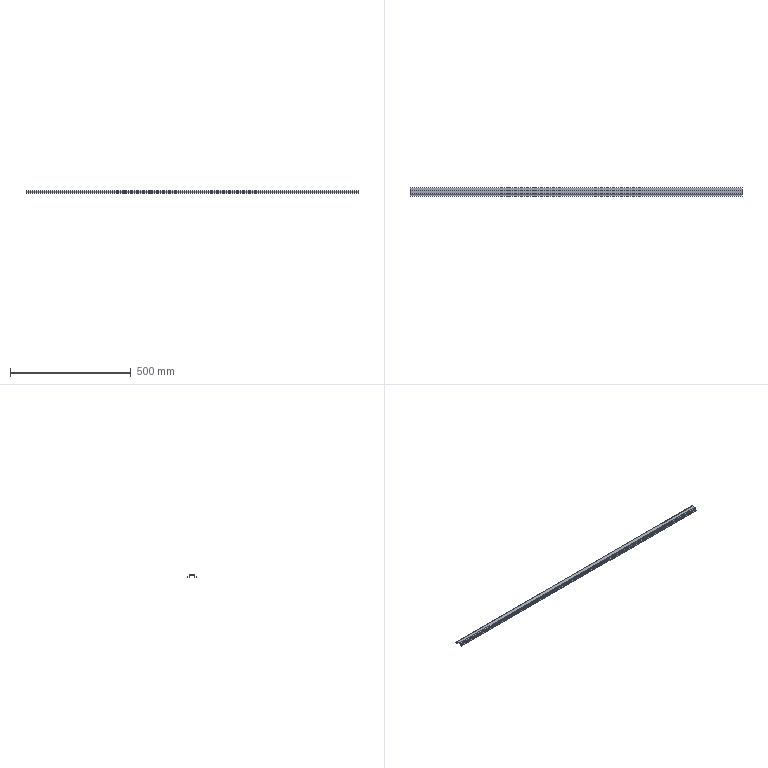Part | SolidWorks | features EdgeFlange 2, FlatPattern 1, SMBaseFlange 1, SheetMetal 1 | 1 solid | 38 faces | box 1375 x 34 x 11 mm | volume 101345 mm3 | plane 30 | cylinder 8 | commonest cylinder face diameters 3 x4 6 x4
STEP:
#1=CARTESIAN_POINT('',(687.5,-7.5,0.));
#2=VERTEX_POINT('',#1);
#3=CARTESIAN_POINT('',(687.5,7.5,0.));
#4=VERTEX_POINT('',#3);
#5=CARTESIAN_POINT('',(687.5,-7.5,0.));
#6=DIRECTION('',(0.,1.,0.));
#7=VECTOR('',#6,1000.);
#8=LINE('',#5,#7);
#9=EDGE_CURVE('',#2,#4,#8,.T.);
#10=ORIENTED_EDGE('',*,*,#9,.F.);
#11=CARTESIAN_POINT('',(687.5,-7.5,-1.5));
#12=VERTEX_POINT('',#11);
#13=CARTESIAN_POINT('',(687.5,-7.5,-1.5));
#14=DIRECTION('',(0.,0.,1.));
#15=VECTOR('',#14,1000.);
#16=LINE('',#13,#15);
#17=EDGE_CURVE('',#12,#2,#16,.T.);
#18=ORIENTED_EDGE('',*,*,#17,.F.);
#19=CARTESIAN_POINT('',(687.5,7.5,-1.5));
#20=VERTEX_POINT('',#19);
#21=CARTESIAN_POINT('',(687.5,-7.5,-1.5));
#22=DIRECTION('',(0.,1.,0.));
#23=VECTOR('',#22,1000.);
#24=LINE('',#21,#23);
#25=EDGE_CURVE('',#12,#20,#24,.T.);
#26=ORIENTED_EDGE('',*,*,#25,.T.);
#27=CARTESIAN_POINT('',(687.5,7.5,-1.5));
#28=DIRECTION('',(0.,0.,1.));
#29=VECTOR('',#28,1000.);
#30=LINE('',#27,#29);
#31=EDGE_CURVE('',#20,#4,#30,.T.);
#32=ORIENTED_EDGE('',*,*,#31,.T.);
#33=EDGE_LOOP('',(#10,#18,#26,#32));
#34=FACE_OUTER_BOUND('',#33,.T.);
#35=CARTESIAN_POINT('',(687.5,-7.5,-1.5));
#36=DIRECTION('',(1.,0.,0.));
#37=DIRECTION('',(0.,0.,-1.));
#38=AXIS2_PLACEMENT_3D('',#35,#36,#37);
#39=PLANE('',#38);
#40=ADVANCED_FACE('',(#34),#39,.T.);
#41=CARTESIAN_POINT('',(-687.5,7.5,0.));
#42=VERTEX_POINT('',#41);
#43=CARTESIAN_POINT('',(-687.5,-7.5,0.));
#44=VERTEX_POINT('',#43);
#45=CARTESIAN_POINT('',(-687.5,-7.5,0.));
#46=DIRECTION('',(0.,-1.,0.));
#47=VECTOR('',#46,1000.);
#48=LINE('',#45,#47);
#49=EDGE_CURVE('',#42,#44,#48,.T.);
#50=ORIENTED_EDGE('',*,*,#49,.F.);
#51=CARTESIAN_POINT('',(-687.5,7.5,-1.5));
#52=VERTEX_POINT('',#51);
#53=CARTESIAN_POINT('',(-687.5,7.5,-1.5));
#54=DIRECTION('',(0.,0.,1.));
#55=VECTOR('',#54,1000.);
#56=LINE('',#53,#55);
#57=EDGE_CURVE('',#52,#42,#56,.T.);
#58=ORIENTED_EDGE('',*,*,#57,.F.);
#59=CARTESIAN_POINT('',(-687.5,-7.5,-1.5));
#60=VERTEX_POINT('',#59);
#61=CARTESIAN_POINT('',(-687.5,-7.5,-1.5));
#62=DIRECTION('',(0.,-1.,0.));
#63=VECTOR('',#62,1000.);
#64=LINE('',#61,#63);
#65=EDGE_CURVE('',#52,#60,#64,.T.);
#66=ORIENTED_EDGE('',*,*,#65,.T.);
#67=CARTESIAN_POINT('',(-687.5,-7.5,-1.5));
#68=DIRECTION('',(0.,0.,1.));
#69=VECTOR('',#68,1000.);
#70=LINE('',#67,#69);
#71=EDGE_CURVE('',#60,#44,#70,.T.);
#72=ORIENTED_EDGE('',*,*,#71,.T.);
#73=EDGE_LOOP('',(#50,#58,#66,#72));
#74=FACE_OUTER_BOUND('',#73,.T.);
#75=CARTESIAN_POINT('',(-687.5,-7.5,-1.5));
#76=DIRECTION('',(-1.,0.,0.));
#77=DIRECTION('',(0.,0.,1.));
#78=AXIS2_PLACEMENT_3D('',#75,#76,#77);
#79=PLANE('',#78);
#80=ADVANCED_FACE('',(#74),#79,.T.);
#81=ORIENTED_EDGE('',*,*,#25,.F.);
#82=CARTESIAN_POINT('',(-687.5,-7.5,-1.5));
#83=DIRECTION('',(1.,0.,0.));
#84=VECTOR('',#83,1000.);
#85=LINE('',#82,#84);
#86=EDGE_CURVE('',#60,#12,#85,.T.);
#87=ORIENTED_EDGE('',*,*,#86,.F.);
#88=ORIENTED_EDGE('',*,*,#65,.F.);
#89=CARTESIAN_POINT('',(-687.5,7.5,-1.5));
#90=DIRECTION('',(-1.,0.,0.));
#91=VECTOR('',#90,1000.);
#92=LINE('',#89,#91);
#93=EDGE_CURVE('',#20,#52,#92,.T.);
#94=ORIENTED_EDGE('',*,*,#93,.F.);
#95=EDGE_LOOP('',(#81,#87,#88,#94));
#96=FACE_OUTER_BOUND('',#95,.T.);
#97=CARTESIAN_POINT('',(0.,0.,-1.5));
#98=DIRECTION('',(0.,0.,-1.));
#99=DIRECTION('',(-1.,0.,0.));
#100=AXIS2_PLACEMENT_3D('',#97,#98,#99);
#101=PLANE('',#100);
#102=ADVANCED_FACE('',(#96),#101,.T.);
#103=ORIENTED_EDGE('',*,*,#9,.T.);
#104=CARTESIAN_POINT('',(-687.5,7.5,0.));
#105=DIRECTION('',(-1.,0.,0.));
#106=VECTOR('',#105,1000.);
#107=LINE('',#104,#106);
#108=EDGE_CURVE('',#4,#42,#107,.T.);
#109=ORIENTED_EDGE('',*,*,#108,.T.);
#110=ORIENTED_EDGE('',*,*,#49,.T.);
#111=CARTESIAN_POINT('',(-687.5,-7.5,0.));
#112=DIRECTION('',(1.,0.,0.));
#113=VECTOR('',#112,1000.);
#114=LINE('',#111,#113);
#115=EDGE_CURVE('',#44,#2,#114,.T.);
#116=ORIENTED_EDGE('',*,*,#115,.T.);
#117=EDGE_LOOP('',(#103,#109,#110,#116));
#118=FACE_OUTER_BOUND('',#117,.T.);
#119=CARTESIAN_POINT('',(0.,0.,0.));
#120=DIRECTION('',(0.,0.,-1.));
#121=DIRECTION('',(-1.,0.,0.));
#122=AXIS2_PLACEMENT_3D('',#119,#120,#121);
#123=PLANE('',#122);
#124=ADVANCED_FACE('',(#118),#123,.F.);
#125=CARTESIAN_POINT('',(-687.5,9.,-3.));
#126=VERTEX_POINT('',#125);
#127=CARTESIAN_POINT('',(-687.5,10.5,-3.));
#128=VERTEX_POINT('',#127);
#129=CARTESIAN_POINT('',(-687.5,10.5,-3.));
#130=DIRECTION('',(0.,1.,0.));
#131=VECTOR('',#130,1000.);
#132=LINE('',#129,#131);
#133=EDGE_CURVE('',#126,#128,#132,.T.);
#134=ORIENTED_EDGE('',*,*,#133,.F.);
#135=CARTESIAN_POINT('',(-687.5,7.5,-3.));
#136=DIRECTION('',(-1.,0.,0.));
#137=DIRECTION('',(0.,0.,-1.));
#138=AXIS2_PLACEMENT_3D('',#135,#136,#137);
#139=CIRCLE('',#138,1.5);
#140=EDGE_CURVE('',#52,#126,#139,.T.);
#141=ORIENTED_EDGE('',*,*,#140,.F.);
#142=ORIENTED_EDGE('',*,*,#57,.T.);
#143=CARTESIAN_POINT('',(-687.5,7.5,-3.));
#144=DIRECTION('',(-1.,0.,0.));
#145=DIRECTION('',(0.,0.,-1.));
#146=AXIS2_PLACEMENT_3D('',#143,#144,#145);
#147=CIRCLE('',#146,3.);
#148=EDGE_CURVE('',#42,#128,#147,.T.);
#149=ORIENTED_EDGE('',*,*,#148,.T.);
#150=EDGE_LOOP('',(#134,#141,#142,#149));
#151=FACE_OUTER_BOUND('',#150,.T.);
#152=CARTESIAN_POINT('',(-687.5,7.5,-3.));
#153=DIRECTION('',(-1.,0.,0.));
#154=DIRECTION('',(0.,0.,1.));
#155=AXIS2_PLACEMENT_3D('',#152,#153,#154);
#156=PLANE('',#155);
#157=ADVANCED_FACE('',(#151),#156,.T.);
#158=CARTESIAN_POINT('',(687.5,9.,-3.));
#159=VERTEX_POINT('',#158);
#160=CARTESIAN_POINT('',(687.5,7.5,-3.));
#161=DIRECTION('',(1.,0.,0.));
#162=DIRECTION('',(0.,0.,-1.));
#163=AXIS2_PLACEMENT_3D('',#160,#161,#162);
#164=CIRCLE('',#163,1.5);
#165=EDGE_CURVE('',#159,#20,#164,.T.);
#166=ORIENTED_EDGE('',*,*,#165,.F.);
#167=CARTESIAN_POINT('',(687.5,10.5,-3.));
#168=VERTEX_POINT('',#167);
#169=CARTESIAN_POINT('',(687.5,9.,-3.));
#170=DIRECTION('',(0.,1.,0.));
#171=VECTOR('',#170,1000.);
#172=LINE('',#169,#171);
#173=EDGE_CURVE('',#159,#168,#172,.T.);
#174=ORIENTED_EDGE('',*,*,#173,.T.);
#175=CARTESIAN_POINT('',(687.5,7.5,-3.));
#176=DIRECTION('',(1.,0.,0.));
#177=DIRECTION('',(0.,0.,-1.));
#178=AXIS2_PLACEMENT_3D('',#175,#176,#177);
#179=CIRCLE('',#178,3.);
#180=EDGE_CURVE('',#168,#4,#179,.T.);
#181=ORIENTED_EDGE('',*,*,#180,.T.);
#182=ORIENTED_EDGE('',*,*,#31,.F.);
#183=EDGE_LOOP('',(#166,#174,#181,#182));
#184=FACE_OUTER_BOUND('',#183,.T.);
#185=CARTESIAN_POINT('',(687.5,7.5,-3.));
#186=DIRECTION('',(-1.,0.,0.));
#187=DIRECTION('',(0.,0.,1.));
#188=AXIS2_PLACEMENT_3D('',#185,#186,#187);
#189=PLANE('',#188);
#190=ADVANCED_FACE('',(#184),#189,.F.);
#191=ORIENTED_EDGE('',*,*,#108,.F.);
#192=ORIENTED_EDGE('',*,*,#180,.F.);
#193=CARTESIAN_POINT('',(-687.5,10.5,-3.));
#194=DIRECTION('',(-1.,0.,0.));
#195=VECTOR('',#194,1000.);
#196=LINE('',#193,#195);
#197=EDGE_CURVE('',#168,#128,#196,.T.);
#198=ORIENTED_EDGE('',*,*,#197,.T.);
#199=ORIENTED_EDGE('',*,*,#148,.F.);
#200=EDGE_LOOP('',(#191,#192,#198,#199));
#201=FACE_OUTER_BOUND('',#200,.T.);
#202=CARTESIAN_POINT('',(687.5,7.5,-3.));
#203=DIRECTION('',(1.,0.,0.));
#204=DIRECTION('',(0.,1.,0.));
#205=AXIS2_PLACEMENT_3D('',#202,#203,#204);
#206=CYLINDRICAL_SURFACE('',#205,3.);
#207=ADVANCED_FACE('',(#201),#206,.T.);
#208=ORIENTED_EDGE('',*,*,#93,.T.);
#209=ORIENTED_EDGE('',*,*,#140,.T.);
#210=CARTESIAN_POINT('',(-687.5,9.,-3.));
#211=DIRECTION('',(1.,0.,0.));
#212=VECTOR('',#211,1000.);
#213=LINE('',#210,#212);
#214=EDGE_CURVE('',#126,#159,#213,.T.);
#215=ORIENTED_EDGE('',*,*,#214,.T.);
#216=ORIENTED_EDGE('',*,*,#165,.T.);
#217=EDGE_LOOP('',(#208,#209,#215,#216));
#218=FACE_OUTER_BOUND('',#217,.T.);
#219=CARTESIAN_POINT('',(687.5,7.5,-3.));
#220=DIRECTION('',(1.,0.,0.));
#221=DIRECTION('',(0.,1.,0.));
#222=AXIS2_PLACEMENT_3D('',#219,#220,#221);
#223=CYLINDRICAL_SURFACE('',#222,1.5);
#224=ADVANCED_FACE('',(#218),#223,.F.);
#225=ORIENTED_EDGE('',*,*,#173,.F.);
#226=CARTESIAN_POINT('',(687.5,9.,-8.));
#227=VERTEX_POINT('',#226);
#228=CARTESIAN_POINT('',(687.5,9.,-8.));
#229=DIRECTION('',(0.,0.,-1.));
#230=VECTOR('',#229,1000.);
#231=LINE('',#228,#230);
#232=EDGE_CURVE('',#159,#227,#231,.T.);
#233=ORIENTED_EDGE('',*,*,#232,.T.);
#234=CARTESIAN_POINT('',(687.5,10.5,-8.));
#235=VERTEX_POINT('',#234);
#236=CARTESIAN_POINT('',(687.5,10.5,-8.));
#237=DIRECTION('',(0.,-1.,0.));
#238=VECTOR('',#237,1000.);
#239=LINE('',#236,#238);
#240=EDGE_CURVE('',#235,#227,#239,.T.);
#241=ORIENTED_EDGE('',*,*,#240,.F.);
#242=CARTESIAN_POINT('',(687.5,10.5,0.));
#243=DIRECTION('',(0.,0.,-1.));
#244=VECTOR('',#243,1000.);
#245=LINE('',#242,#244);
#246=EDGE_CURVE('',#168,#235,#245,.T.);
#247=ORIENTED_EDGE('',*,*,#246,.F.);
#248=EDGE_LOOP('',(#225,#233,#241,#247));
#249=FACE_OUTER_BOUND('',#248,.T.);
#250=CARTESIAN_POINT('',(687.5,10.5,-8.));
#251=DIRECTION('',(-1.,0.,0.));
#252=DIRECTION('',(0.,0.,1.));
#253=AXIS2_PLACEMENT_3D('',#250,#251,#252);
#254=PLANE('',#253);
#255=ADVANCED_FACE('',(#249),#254,.F.);
#256=ORIENTED_EDGE('',*,*,#133,.T.);
#257=CARTESIAN_POINT('',(-687.5,10.5,-8.));
#258=VERTEX_POINT('',#257);
#259=CARTESIAN_POINT('',(-687.5,10.5,0.));
#260=DIRECTION('',(0.,0.,1.));
#261=VECTOR('',#260,1000.);
#262=LINE('',#259,#261);
#263=EDGE_CURVE('',#258,#128,#262,.T.);
#264=ORIENTED_EDGE('',*,*,#263,.F.);
#265=CARTESIAN_POINT('',(-687.5,9.,-8.));
#266=VERTEX_POINT('',#265);
#267=CARTESIAN_POINT('',(-687.5,10.5,-8.));
#268=DIRECTION('',(0.,-1.,0.));
#269=VECTOR('',#268,1000.);
#270=LINE('',#267,#269);
#271=EDGE_CURVE('',#258,#266,#270,.T.);
#272=ORIENTED_EDGE('',*,*,#271,.T.);
#273=CARTESIAN_POINT('',(-687.5,9.,-1.5));
#274=DIRECTION('',(0.,0.,1.));
#275=VECTOR('',#274,1000.);
#276=LINE('',#273,#275);
#277=EDGE_CURVE('',#266,#126,#276,.T.);
#278=ORIENTED_EDGE('',*,*,#277,.T.);
#279=EDGE_LOOP('',(#256,#264,#272,#278));
#280=FACE_OUTER_BOUND('',#279,.T.);
#281=CARTESIAN_POINT('',(-687.5,10.5,-1.5));
#282=DIRECTION('',(1.,0.,0.));
#283=DIRECTION('',(0.,0.,-1.));
#284=AXIS2_PLACEMENT_3D('',#281,#282,#283);
#285=PLANE('',#284);
#286=ADVANCED_FACE('',(#280),#285,.F.);
#287=ORIENTED_EDGE('',*,*,#197,.F.);
#288=ORIENTED_EDGE('',*,*,#246,.T.);
#289=CARTESIAN_POINT('',(0.,10.5,-8.));
#290=DIRECTION('',(-1.,0.,0.));
#291=VECTOR('',#290,1000.);
#292=LINE('',#289,#291);
#293=EDGE_CURVE('',#235,#258,#292,.T.);
#294=ORIENTED_EDGE('',*,*,#293,.T.);
#295=ORIENTED_EDGE('',*,*,#263,.T.);
#296=EDGE_LOOP('',(#287,#288,#294,#295));
#297=FACE_OUTER_BOUND('',#296,.T.);
#298=CARTESIAN_POINT('',(0.,10.5,0.));
#299=DIRECTION('',(0.,-1.,0.));
#300=DIRECTION('',(0.,0.,-1.));
#301=AXIS2_PLACEMENT_3D('',#298,#299,#300);
#302=PLANE('',#301);
#303=ADVANCED_FACE('',(#297),#302,.F.);
#304=ORIENTED_EDGE('',*,*,#232,.F.);
#305=ORIENTED_EDGE('',*,*,#214,.F.);
#306=ORIENTED_EDGE('',*,*,#277,.F.);
#307=CARTESIAN_POINT('',(-687.5,9.,-8.));
#308=DIRECTION('',(-1.,0.,0.));
#309=VECTOR('',#308,1000.);
#310=LINE('',#307,#309);
#311=EDGE_CURVE('',#227,#266,#310,.T.);
#312=ORIENTED_EDGE('',*,*,#311,.F.);
#313=EDGE_LOOP('',(#304,#305,#306,#312));
#314=FACE_OUTER_BOUND('',#313,.T.);
#315=CARTESIAN_POINT('',(0.,9.,0.));
#316=DIRECTION('',(0.,-1.,0.));
#317=DIRECTION('',(0.,0.,-1.));
#318=AXIS2_PLACEMENT_3D('',#315,#316,#317);
#319=PLANE('',#318);
#320=ADVANCED_FACE('',(#314),#319,.T.);
#321=CARTESIAN_POINT('',(687.5,-9.,-3.));
#322=VERTEX_POINT('',#321);
#323=CARTESIAN_POINT('',(687.5,-10.5,-3.));
#324=VERTEX_POINT('',#323);
#325=CARTESIAN_POINT('',(687.5,-10.5,-3.));
#326=DIRECTION('',(0.,-1.,0.));
#327=VECTOR('',#326,1000.);
#328=LINE('',#325,#327);
#329=EDGE_CURVE('',#322,#324,#328,.T.);
#330=ORIENTED_EDGE('',*,*,#329,.F.);
#331=CARTESIAN_POINT('',(687.5,-7.5,-3.));
#332=DIRECTION('',(1.,0.,0.));
#333=DIRECTION('',(0.,0.,1.));
#334=AXIS2_PLACEMENT_3D('',#331,#332,#333);
#335=CIRCLE('',#334,1.5);
#336=EDGE_CURVE('',#12,#322,#335,.T.);
#337=ORIENTED_EDGE('',*,*,#336,.F.);
#338=ORIENTED_EDGE('',*,*,#17,.T.);
#339=CARTESIAN_POINT('',(687.5,-7.5,-3.));
#340=DIRECTION('',(1.,0.,0.));
#341=DIRECTION('',(0.,0.,1.));
#342=AXIS2_PLACEMENT_3D('',#339,#340,#341);
#343=CIRCLE('',#342,3.);
#344=EDGE_CURVE('',#2,#324,#343,.T.);
#345=ORIENTED_EDGE('',*,*,#344,.T.);
#346=EDGE_LOOP('',(#330,#337,#338,#345));
#347=FACE_OUTER_BOUND('',#346,.T.);
#348=CARTESIAN_POINT('',(687.5,-7.5,-3.));
#349=DIRECTION('',(1.,0.,0.));
#350=DIRECTION('',(0.,0.,-1.));
#351=AXIS2_PLACEMENT_3D('',#348,#349,#350);
#352=PLANE('',#351);
#353=ADVANCED_FACE('',(#347),#352,.T.);
#354=CARTESIAN_POINT('',(-687.5,-9.,-3.));
#355=VERTEX_POINT('',#354);
#356=CARTESIAN_POINT('',(-687.5,-7.5,-3.));
#357=DIRECTION('',(-1.,0.,0.));
#358=DIRECTION('',(0.,0.,1.));
#359=AXIS2_PLACEMENT_3D('',#356,#357,#358);
#360=CIRCLE('',#359,1.5);
#361=EDGE_CURVE('',#355,#60,#360,.T.);
#362=ORIENTED_EDGE('',*,*,#361,.F.);
#363=CARTESIAN_POINT('',(-687.5,-10.5,-3.));
#364=VERTEX_POINT('',#363);
#365=CARTESIAN_POINT('',(-687.5,-9.,-3.));
#366=DIRECTION('',(0.,-1.,0.));
#367=VECTOR('',#366,1000.);
#368=LINE('',#365,#367);
#369=EDGE_CURVE('',#355,#364,#368,.T.);
#370=ORIENTED_EDGE('',*,*,#369,.T.);
#371=CARTESIAN_POINT('',(-687.5,-7.5,-3.));
#372=DIRECTION('',(-1.,0.,0.));
#373=DIRECTION('',(0.,0.,1.));
#374=AXIS2_PLACEMENT_3D('',#371,#372,#373);
#375=CIRCLE('',#374,3.);
#376=EDGE_CURVE('',#364,#44,#375,.T.);
#377=ORIENTED_EDGE('',*,*,#376,.T.);
#378=ORIENTED_EDGE('',*,*,#71,.F.);
#379=EDGE_LOOP('',(#362,#370,#377,#378));
#380=FACE_OUTER_BOUND('',#379,.T.);
#381=CARTESIAN_POINT('',(-687.5,-7.5,-3.));
#382=DIRECTION('',(1.,0.,0.));
#383=DIRECTION('',(0.,0.,-1.));
#384=AXIS2_PLACEMENT_3D('',#381,#382,#383);
#385=PLANE('',#384);
#386=ADVANCED_FACE('',(#380),#385,.F.);
#387=ORIENTED_EDGE('',*,*,#115,.F.);
#388=ORIENTED_EDGE('',*,*,#376,.F.);
#389=CARTESIAN_POINT('',(687.5,-10.5,-3.));
#390=DIRECTION('',(1.,0.,0.));
#391=VECTOR('',#390,1000.);
#392=LINE('',#389,#391);
#393=EDGE_CURVE('',#364,#324,#392,.T.);
#394=ORIENTED_EDGE('',*,*,#393,.T.);
#395=ORIENTED_EDGE('',*,*,#344,.F.);
#396=EDGE_LOOP('',(#387,#388,#394,#395));
#397=FACE_OUTER_BOUND('',#396,.T.);
#398=CARTESIAN_POINT('',(-687.5,-7.5,-3.));
#399=DIRECTION('',(-1.,0.,0.));
#400=DIRECTION('',(0.,-1.,0.));
#401=AXIS2_PLACEMENT_3D('',#398,#399,#400);
#402=CYLINDRICAL_SURFACE('',#401,3.);
#403=ADVANCED_FACE('',(#397),#402,.T.);
#404=ORIENTED_EDGE('',*,*,#86,.T.);
#405=ORIENTED_EDGE('',*,*,#336,.T.);
#406=CARTESIAN_POINT('',(687.5,-9.,-3.));
#407=DIRECTION('',(-1.,0.,0.));
#408=VECTOR('',#407,1000.);
#409=LINE('',#406,#408);
#410=EDGE_CURVE('',#322,#355,#409,.T.);
#411=ORIENTED_EDGE('',*,*,#410,.T.);
#412=ORIENTED_EDGE('',*,*,#361,.T.);
#413=EDGE_LOOP('',(#404,#405,#411,#412));
#414=FACE_OUTER_BOUND('',#413,.T.);
#415=CARTESIAN_POINT('',(-687.5,-7.5,-3.));
#416=DIRECTION('',(-1.,0.,0.));
#417=DIRECTION('',(0.,-1.,0.));
#418=AXIS2_PLACEMENT_3D('',#415,#416,#417);
#419=CYLINDRICAL_SURFACE('',#418,1.5);
#420=ADVANCED_FACE('',(#414),#419,.F.);
#421=ORIENTED_EDGE('',*,*,#369,.F.);
#422=CARTESIAN_POINT('',(-687.5,-9.,-8.));
#423=VERTEX_POINT('',#422);
#424=CARTESIAN_POINT('',(-687.5,-9.,-8.));
#425=DIRECTION('',(0.,0.,-1.));
#426=VECTOR('',#425,1000.);
#427=LINE('',#424,#426);
#428=EDGE_CURVE('',#355,#423,#427,.T.);
#429=ORIENTED_EDGE('',*,*,#428,.T.);
#430=CARTESIAN_POINT('',(-687.5,-10.5,-8.));
#431=VERTEX_POINT('',#430);
#432=CARTESIAN_POINT('',(-687.5,-10.5,-8.));
#433=DIRECTION('',(0.,1.,0.));
#434=VECTOR('',#433,1000.);
#435=LINE('',#432,#434);
#436=EDGE_CURVE('',#431,#423,#435,.T.);
#437=ORIENTED_EDGE('',*,*,#436,.F.);
#438=CARTESIAN_POINT('',(-687.5,-10.5,0.));
#439=DIRECTION('',(0.,0.,-1.));
#440=VECTOR('',#439,1000.);
#441=LINE('',#438,#440);
#442=EDGE_CURVE('',#364,#431,#441,.T.);
#443=ORIENTED_EDGE('',*,*,#442,.F.);
#444=EDGE_LOOP('',(#421,#429,#437,#443));
#445=FACE_OUTER_BOUND('',#444,.T.);
#446=CARTESIAN_POINT('',(-687.5,-10.5,-8.));
#447=DIRECTION('',(1.,0.,0.));
#448=DIRECTION('',(0.,0.,-1.));
#449=AXIS2_PLACEMENT_3D('',#446,#447,#448);
#450=PLANE('',#449);
#451=ADVANCED_FACE('',(#445),#450,.F.);
#452=ORIENTED_EDGE('',*,*,#329,.T.);
#453=CARTESIAN_POINT('',(687.5,-10.5,-8.));
#454=VERTEX_POINT('',#453);
#455=CARTESIAN_POINT('',(687.5,-10.5,0.));
#456=DIRECTION('',(0.,0.,1.));
#457=VECTOR('',#456,1000.);
#458=LINE('',#455,#457);
#459=EDGE_CURVE('',#454,#324,#458,.T.);
#460=ORIENTED_EDGE('',*,*,#459,.F.);
#461=CARTESIAN_POINT('',(687.5,-9.,-8.));
#462=VERTEX_POINT('',#461);
#463=CARTESIAN_POINT('',(687.5,-10.5,-8.));
#464=DIRECTION('',(0.,1.,0.));
#465=VECTOR('',#464,1000.);
#466=LINE('',#463,#465);
#467=EDGE_CURVE('',#454,#462,#466,.T.);
#468=ORIENTED_EDGE('',*,*,#467,.T.);
#469=CARTESIAN_POINT('',(687.5,-9.,-1.5));
#470=DIRECTION('',(0.,0.,1.));
#471=VECTOR('',#470,1000.);
#472=LINE('',#469,#471);
#473=EDGE_CURVE('',#462,#322,#472,.T.);
#474=ORIENTED_EDGE('',*,*,#473,.T.);
#475=EDGE_LOOP('',(#452,#460,#468,#474));
#476=FACE_OUTER_BOUND('',#475,.T.);
#477=CARTESIAN_POINT('',(687.5,-10.5,-1.5));
#478=DIRECTION('',(-1.,0.,0.));
#479=DIRECTION('',(0.,0.,1.));
#480=AXIS2_PLACEMENT_3D('',#477,#478,#479);
#481=PLANE('',#480);
#482=ADVANCED_FACE('',(#476),#481,.F.);
#483=ORIENTED_EDGE('',*,*,#393,.F.);
#484=ORIENTED_EDGE('',*,*,#442,.T.);
#485=CARTESIAN_POINT('',(0.,-10.5,-8.));
#486=DIRECTION('',(1.,0.,0.));
#487=VECTOR('',#486,1000.);
#488=LINE('',#485,#487);
#489=EDGE_CURVE('',#431,#454,#488,.T.);
#490=ORIENTED_EDGE('',*,*,#489,.T.);
#491=ORIENTED_EDGE('',*,*,#459,.T.);
#492=EDGE_LOOP('',(#483,#484,#490,#491));
#493=FACE_OUTER_BOUND('',#492,.T.);
#494=CARTESIAN_POINT('',(0.,-10.5,0.));
#495=DIRECTION('',(0.,1.,0.));
#496=DIRECTION('',(0.,0.,1.));
#497=AXIS2_PLACEMENT_3D('',#494,#495,#496);
#498=PLANE('',#497);
#499=ADVANCED_FACE('',(#493),#498,.F.);
#500=ORIENTED_EDGE('',*,*,#428,.F.);
#501=ORIENTED_EDGE('',*,*,#410,.F.);
#502=ORIENTED_EDGE('',*,*,#473,.F.);
#503=CARTESIAN_POINT('',(687.5,-9.,-8.));
#504=DIRECTION('',(1.,0.,0.));
#505=VECTOR('',#504,1000.);
#506=LINE('',#503,#505);
#507=EDGE_CURVE('',#423,#462,#506,.T.);
#508=ORIENTED_EDGE('',*,*,#507,.F.);
#509=EDGE_LOOP('',(#500,#501,#502,#508));
#510=FACE_OUTER_BOUND('',#509,.T.);
#511=CARTESIAN_POINT('',(0.,-9.,0.));
#512=DIRECTION('',(0.,1.,0.));
#513=DIRECTION('',(0.,0.,1.));
#514=AXIS2_PLACEMENT_3D('',#511,#512,#513);
#515=PLANE('',#514);
#516=ADVANCED_FACE('',(#510),#515,.T.);
#517=CARTESIAN_POINT('',(687.5,12.,-9.5));
#518=VERTEX_POINT('',#517);
#519=CARTESIAN_POINT('',(687.5,12.,-11.));
#520=VERTEX_POINT('',#519);
#521=CARTESIAN_POINT('',(687.5,12.,-11.));
#522=DIRECTION('',(0.,0.,-1.));
#523=VECTOR('',#522,1000.);
#524=LINE('',#521,#523);
#525=EDGE_CURVE('',#518,#520,#524,.T.);
#526=ORIENTED_EDGE('',*,*,#525,.F.);
#527=CARTESIAN_POINT('',(687.5,12.,-8.));
#528=DIRECTION('',(1.,0.,0.));
#529=DIRECTION('',(0.,0.,1.));
#530=AXIS2_PLACEMENT_3D('',#527,#528,#529);
#531=CIRCLE('',#530,1.5);
#532=EDGE_CURVE('',#235,#518,#531,.T.);
#533=ORIENTED_EDGE('',*,*,#532,.F.);
#534=ORIENTED_EDGE('',*,*,#240,.T.);
#535=CARTESIAN_POINT('',(687.5,12.,-8.));
#536=DIRECTION('',(1.,0.,0.));
#537=DIRECTION('',(0.,0.,1.));
#538=AXIS2_PLACEMENT_3D('',#535,#536,#537);
#539=CIRCLE('',#538,3.);
#540=EDGE_CURVE('',#227,#520,#539,.T.);
#541=ORIENTED_EDGE('',*,*,#540,.T.);
#542=EDGE_LOOP('',(#526,#533,#534,#541));
#543=FACE_OUTER_BOUND('',#542,.T.);
#544=CARTESIAN_POINT('',(687.5,12.,-8.));
#545=DIRECTION('',(1.,0.,0.));
#546=DIRECTION('',(0.,0.,-1.));
#547=AXIS2_PLACEMENT_3D('',#544,#545,#546);
#548=PLANE('',#547);
#549=ADVANCED_FACE('',(#543),#548,.T.);
#550=CARTESIAN_POINT('',(-687.5,12.,-9.5));
#551=VERTEX_POINT('',#550);
#552=CARTESIAN_POINT('',(-687.5,12.,-8.));
#553=DIRECTION('',(-1.,0.,0.));
#554=DIRECTION('',(0.,0.,1.));
#555=AXIS2_PLACEMENT_3D('',#552,#553,#554);
#556=CIRCLE('',#555,1.5);
#557=EDGE_CURVE('',#551,#258,#556,.T.);
#558=ORIENTED_EDGE('',*,*,#557,.F.);
#559=CARTESIAN_POINT('',(-687.5,12.,-11.));
#560=VERTEX_POINT('',#559);
#561=CARTESIAN_POINT('',(-687.5,12.,-9.5));
#562=DIRECTION('',(0.,0.,-1.));
#563=VECTOR('',#562,1000.);
#564=LINE('',#561,#563);
#565=EDGE_CURVE('',#551,#560,#564,.T.);
#566=ORIENTED_EDGE('',*,*,#565,.T.);
#567=CARTESIAN_POINT('',(-687.5,12.,-8.));
#568=DIRECTION('',(-1.,0.,0.));
#569=DIRECTION('',(0.,0.,1.));
#570=AXIS2_PLACEMENT_3D('',#567,#568,#569);
#571=CIRCLE('',#570,3.);
#572=EDGE_CURVE('',#560,#266,#571,.T.);
#573=ORIENTED_EDGE('',*,*,#572,.T.);
#574=ORIENTED_EDGE('',*,*,#271,.F.);
#575=EDGE_LOOP('',(#558,#566,#573,#574));
#576=FACE_OUTER_BOUND('',#575,.T.);
#577=CARTESIAN_POINT('',(-687.5,12.,-8.));
#578=DIRECTION('',(1.,0.,0.));
#579=DIRECTION('',(0.,0.,-1.));
#580=AXIS2_PLACEMENT_3D('',#577,#578,#579);
#581=PLANE('',#580);
#582=ADVANCED_FACE('',(#576),#581,.F.);
#583=ORIENTED_EDGE('',*,*,#311,.T.);
#584=ORIENTED_EDGE('',*,*,#572,.F.);
#585=CARTESIAN_POINT('',(0.,12.,-11.));
#586=DIRECTION('',(-1.,0.,0.));
#587=VECTOR('',#586,1000.);
#588=LINE('',#585,#587);
#589=EDGE_CURVE('',#520,#560,#588,.T.);
#590=ORIENTED_EDGE('',*,*,#589,.F.);
#591=ORIENTED_EDGE('',*,*,#540,.F.);
#592=EDGE_LOOP('',(#583,#584,#590,#591));
#593=FACE_OUTER_BOUND('',#592,.T.);
#594=CARTESIAN_POINT('',(-687.5,12.,-8.));
#595=DIRECTION('',(-1.,0.,0.));
#596=DIRECTION('',(0.,0.,-1.));
#597=AXIS2_PLACEMENT_3D('',#594,#595,#596);
#598=CYLINDRICAL_SURFACE('',#597,3.);
#599=ADVANCED_FACE('',(#593),#598,.T.);
#600=ORIENTED_EDGE('',*,*,#293,.F.);
#601=ORIENTED_EDGE('',*,*,#532,.T.);
#602=CARTESIAN_POINT('',(687.5,12.,-9.5));
#603=DIRECTION('',(-1.,0.,0.));
#604=VECTOR('',#603,1000.);
#605=LINE('',#602,#604);
#606=EDGE_CURVE('',#518,#551,#605,.T.);
#607=ORIENTED_EDGE('',*,*,#606,.T.);
#608=ORIENTED_EDGE('',*,*,#557,.T.);
#609=EDGE_LOOP('',(#600,#601,#607,#608));
#610=FACE_OUTER_BOUND('',#609,.T.);
#611=CARTESIAN_POINT('',(-687.5,12.,-8.));
#612=DIRECTION('',(-1.,0.,0.));
#613=DIRECTION('',(0.,0.,-1.));
#614=AXIS2_PLACEMENT_3D('',#611,#612,#613);
#615=CYLINDRICAL_SURFACE('',#614,1.5);
#616=ADVANCED_FACE('',(#610),#615,.F.);
#617=CARTESIAN_POINT('',(-687.5,17.,-11.));
#618=VERTEX_POINT('',#617);
#619=CARTESIAN_POINT('',(-687.5,10.5,-11.));
#620=DIRECTION('',(0.,-1.,0.));
#621=VECTOR('',#620,1000.);
#622=LINE('',#619,#621);
#623=EDGE_CURVE('',#618,#560,#622,.T.);
#624=ORIENTED_EDGE('',*,*,#623,.T.);
#625=ORIENTED_EDGE('',*,*,#565,.F.);
#626=CARTESIAN_POINT('',(-687.5,17.,-9.5));
#627=VERTEX_POINT('',#626);
#628=CARTESIAN_POINT('',(-687.5,0.,-9.5));
#629=DIRECTION('',(0.,-1.,0.));
#630=VECTOR('',#629,1000.);
#631=LINE('',#628,#630);
#632=EDGE_CURVE('',#627,#551,#631,.T.);
#633=ORIENTED_EDGE('',*,*,#632,.F.);
#634=CARTESIAN_POINT('',(-687.5,17.,-11.));
#635=DIRECTION('',(0.,0.,1.));
#636=VECTOR('',#635,1000.);
#637=LINE('',#634,#636);
#638=EDGE_CURVE('',#618,#627,#637,.T.);
#639=ORIENTED_EDGE('',*,*,#638,.F.);
#640=EDGE_LOOP('',(#624,#625,#633,#639));
#641=FACE_OUTER_BOUND('',#640,.T.);
#642=CARTESIAN_POINT('',(-687.5,10.5,-11.));
#643=DIRECTION('',(-1.,0.,0.));
#644=DIRECTION('',(0.,0.,1.));
#645=AXIS2_PLACEMENT_3D('',#642,#643,#644);
#646=PLANE('',#645);
#647=ADVANCED_FACE('',(#641),#646,.T.);
#648=CARTESIAN_POINT('',(687.5,17.,-9.5));
#649=VERTEX_POINT('',#648);
#650=CARTESIAN_POINT('',(687.5,0.,-9.5));
#651=DIRECTION('',(0.,1.,0.));
#652=VECTOR('',#651,1000.);
#653=LINE('',#650,#652);
#654=EDGE_CURVE('',#518,#649,#653,.T.);
#655=ORIENTED_EDGE('',*,*,#654,.F.);
#656=ORIENTED_EDGE('',*,*,#525,.T.);
#657=CARTESIAN_POINT('',(687.5,17.,-11.));
#658=VERTEX_POINT('',#657);
#659=CARTESIAN_POINT('',(687.5,17.,-11.));
#660=DIRECTION('',(0.,1.,0.));
#661=VECTOR('',#660,1000.);
#662=LINE('',#659,#661);
#663=EDGE_CURVE('',#520,#658,#662,.T.);
#664=ORIENTED_EDGE('',*,*,#663,.T.);
#665=CARTESIAN_POINT('',(687.5,17.,-11.));
#666=DIRECTION('',(0.,0.,1.));
#667=VECTOR('',#666,1000.);
#668=LINE('',#665,#667);
#669=EDGE_CURVE('',#658,#649,#668,.T.);
#670=ORIENTED_EDGE('',*,*,#669,.T.);
#671=EDGE_LOOP('',(#655,#656,#664,#670));
#672=FACE_OUTER_BOUND('',#671,.T.);
#673=CARTESIAN_POINT('',(687.5,17.,-11.));
#674=DIRECTION('',(1.,0.,0.));
#675=DIRECTION('',(0.,0.,-1.));
#676=AXIS2_PLACEMENT_3D('',#673,#674,#675);
#677=PLANE('',#676);
#678=ADVANCED_FACE('',(#672),#677,.T.);
#679=ORIENTED_EDGE('',*,*,#663,.F.);
#680=ORIENTED_EDGE('',*,*,#589,.T.);
#681=ORIENTED_EDGE('',*,*,#623,.F.);
#682=CARTESIAN_POINT('',(-687.5,17.,-11.));
#683=DIRECTION('',(-1.,0.,0.));
#684=VECTOR('',#683,1000.);
#685=LINE('',#682,#684);
#686=EDGE_CURVE('',#658,#618,#685,.T.);
#687=ORIENTED_EDGE('',*,*,#686,.F.);
#688=EDGE_LOOP('',(#679,#680,#681,#687));
#689=FACE_OUTER_BOUND('',#688,.T.);
#690=CARTESIAN_POINT('',(0.,0.,-11.));
#691=DIRECTION('',(0.,0.,-1.));
#692=DIRECTION('',(-1.,0.,0.));
#693=AXIS2_PLACEMENT_3D('',#690,#691,#692);
#694=PLANE('',#693);
#695=ADVANCED_FACE('',(#689),#694,.T.);
#696=ORIENTED_EDGE('',*,*,#606,.F.);
#697=ORIENTED_EDGE('',*,*,#654,.T.);
#698=CARTESIAN_POINT('',(0.,17.,-9.5));
#699=DIRECTION('',(-1.,0.,0.));
#700=VECTOR('',#699,1000.);
#701=LINE('',#698,#700);
#702=EDGE_CURVE('',#649,#627,#701,.T.);
#703=ORIENTED_EDGE('',*,*,#702,.T.);
#704=ORIENTED_EDGE('',*,*,#632,.T.);
#705=EDGE_LOOP('',(#696,#697,#703,#704));
#706=FACE_OUTER_BOUND('',#705,.T.);
#707=CARTESIAN_POINT('',(0.,0.,-9.5));
#708=DIRECTION('',(0.,0.,-1.));
#709=DIRECTION('',(-1.,0.,0.));
#710=AXIS2_PLACEMENT_3D('',#707,#708,#709);
#711=PLANE('',#710);
#712=ADVANCED_FACE('',(#706),#711,.F.);
#713=ORIENTED_EDGE('',*,*,#702,.F.);
#714=ORIENTED_EDGE('',*,*,#669,.F.);
#715=ORIENTED_EDGE('',*,*,#686,.T.);
#716=ORIENTED_EDGE('',*,*,#638,.T.);
#717=EDGE_LOOP('',(#713,#714,#715,#716));
#718=FACE_OUTER_BOUND('',#717,.T.);
#719=CARTESIAN_POINT('',(-687.5,17.,-11.));
#720=DIRECTION('',(0.,1.,0.));
#721=DIRECTION('',(0.,0.,1.));
#722=AXIS2_PLACEMENT_3D('',#719,#720,#721);
#723=PLANE('',#722);
#724=ADVANCED_FACE('',(#718),#723,.T.);
#725=CARTESIAN_POINT('',(-687.5,-12.,-9.5));
#726=VERTEX_POINT('',#725);
#727=CARTESIAN_POINT('',(-687.5,-12.,-11.));
#728=VERTEX_POINT('',#727);
#729=CARTESIAN_POINT('',(-687.5,-12.,-11.));
#730=DIRECTION('',(0.,0.,-1.));
#731=VECTOR('',#730,1000.);
#732=LINE('',#729,#731);
#733=EDGE_CURVE('',#726,#728,#732,.T.);
#734=ORIENTED_EDGE('',*,*,#733,.F.);
#735=CARTESIAN_POINT('',(-687.5,-12.,-8.));
#736=DIRECTION('',(-1.,0.,0.));
#737=DIRECTION('',(0.,0.,-1.));
#738=AXIS2_PLACEMENT_3D('',#735,#736,#737);
#739=CIRCLE('',#738,1.5);
#740=EDGE_CURVE('',#431,#726,#739,.T.);
#741=ORIENTED_EDGE('',*,*,#740,.F.);
#742=ORIENTED_EDGE('',*,*,#436,.T.);
#743=CARTESIAN_POINT('',(-687.5,-12.,-8.));
#744=DIRECTION('',(-1.,0.,0.));
#745=DIRECTION('',(0.,0.,-1.));
#746=AXIS2_PLACEMENT_3D('',#743,#744,#745);
#747=CIRCLE('',#746,3.);
#748=EDGE_CURVE('',#423,#728,#747,.T.);
#749=ORIENTED_EDGE('',*,*,#748,.T.);
#750=EDGE_LOOP('',(#734,#741,#742,#749));
#751=FACE_OUTER_BOUND('',#750,.T.);
#752=CARTESIAN_POINT('',(-687.5,-12.,-8.));
#753=DIRECTION('',(-1.,0.,0.));
#754=DIRECTION('',(0.,0.,1.));
#755=AXIS2_PLACEMENT_3D('',#752,#753,#754);
#756=PLANE('',#755);
#757=ADVANCED_FACE('',(#751),#756,.T.);
#758=CARTESIAN_POINT('',(687.5,-12.,-9.5));
#759=VERTEX_POINT('',#758);
#760=CARTESIAN_POINT('',(687.5,-12.,-8.));
#761=DIRECTION('',(1.,0.,0.));
#762=DIRECTION('',(0.,0.,-1.));
#763=AXIS2_PLACEMENT_3D('',#760,#761,#762);
#764=CIRCLE('',#763,1.5);
#765=EDGE_CURVE('',#759,#454,#764,.T.);
#766=ORIENTED_EDGE('',*,*,#765,.F.);
#767=CARTESIAN_POINT('',(687.5,-12.,-11.));
#768=VERTEX_POINT('',#767);
#769=CARTESIAN_POINT('',(687.5,-12.,-9.5));
#770=DIRECTION('',(0.,0.,-1.));
#771=VECTOR('',#770,1000.);
#772=LINE('',#769,#771);
#773=EDGE_CURVE('',#759,#768,#772,.T.);
#774=ORIENTED_EDGE('',*,*,#773,.T.);
#775=CARTESIAN_POINT('',(687.5,-12.,-8.));
#776=DIRECTION('',(1.,0.,0.));
#777=DIRECTION('',(0.,0.,-1.));
#778=AXIS2_PLACEMENT_3D('',#775,#776,#777);
#779=CIRCLE('',#778,3.);
#780=EDGE_CURVE('',#768,#462,#779,.T.);
#781=ORIENTED_EDGE('',*,*,#780,.T.);
#782=ORIENTED_EDGE('',*,*,#467,.F.);
#783=EDGE_LOOP('',(#766,#774,#781,#782));
#784=FACE_OUTER_BOUND('',#783,.T.);
#785=CARTESIAN_POINT('',(687.5,-12.,-8.));
#786=DIRECTION('',(-1.,0.,0.));
#787=DIRECTION('',(0.,0.,1.));
#788=AXIS2_PLACEMENT_3D('',#785,#786,#787);
#789=PLANE('',#788);
#790=ADVANCED_FACE('',(#784),#789,.F.);
#791=ORIENTED_EDGE('',*,*,#507,.T.);
#792=ORIENTED_EDGE('',*,*,#780,.F.);
#793=CARTESIAN_POINT('',(-687.5,-12.,-11.));
#794=DIRECTION('',(-1.,0.,0.));
#795=VECTOR('',#794,1000.);
#796=LINE('',#793,#795);
#797=EDGE_CURVE('',#768,#728,#796,.T.);
#798=ORIENTED_EDGE('',*,*,#797,.T.);
#799=ORIENTED_EDGE('',*,*,#748,.F.);
#800=EDGE_LOOP('',(#791,#792,#798,#799));
#801=FACE_OUTER_BOUND('',#800,.T.);
#802=CARTESIAN_POINT('',(687.5,-12.,-8.));
#803=DIRECTION('',(1.,0.,0.));
#804=DIRECTION('',(0.,0.,-1.));
#805=AXIS2_PLACEMENT_3D('',#802,#803,#804);
#806=CYLINDRICAL_SURFACE('',#805,3.);
#807=ADVANCED_FACE('',(#801),#806,.T.);
#808=ORIENTED_EDGE('',*,*,#489,.F.);
#809=ORIENTED_EDGE('',*,*,#740,.T.);
#810=CARTESIAN_POINT('',(-687.5,-12.,-9.5));
#811=DIRECTION('',(1.,0.,0.));
#812=VECTOR('',#811,1000.);
#813=LINE('',#810,#812);
#814=EDGE_CURVE('',#726,#759,#813,.T.);
#815=ORIENTED_EDGE('',*,*,#814,.T.);
#816=ORIENTED_EDGE('',*,*,#765,.T.);
#817=EDGE_LOOP('',(#808,#809,#815,#816));
#818=FACE_OUTER_BOUND('',#817,.T.);
#819=CARTESIAN_POINT('',(687.5,-12.,-8.));
#820=DIRECTION('',(1.,0.,0.));
#821=DIRECTION('',(0.,0.,-1.));
#822=AXIS2_PLACEMENT_3D('',#819,#820,#821);
#823=CYLINDRICAL_SURFACE('',#822,1.5);
#824=ADVANCED_FACE('',(#818),#823,.F.);
#825=CARTESIAN_POINT('',(-687.5,-17.,-9.5));
#826=VERTEX_POINT('',#825);
#827=CARTESIAN_POINT('',(-687.5,0.,-9.5));
#828=DIRECTION('',(0.,-1.,0.));
#829=VECTOR('',#828,1000.);
#830=LINE('',#827,#829);
#831=EDGE_CURVE('',#726,#826,#830,.T.);
#832=ORIENTED_EDGE('',*,*,#831,.F.);
#833=ORIENTED_EDGE('',*,*,#733,.T.);
#834=CARTESIAN_POINT('',(-687.5,-17.,-11.));
#835=VERTEX_POINT('',#834);
#836=CARTESIAN_POINT('',(-687.5,-10.5,-11.));
#837=DIRECTION('',(0.,-1.,0.));
#838=VECTOR('',#837,1000.);
#839=LINE('',#836,#838);
#840=EDGE_CURVE('',#728,#835,#839,.T.);
#841=ORIENTED_EDGE('',*,*,#840,.T.);
#842=CARTESIAN_POINT('',(-687.5,-17.,-11.));
#843=DIRECTION('',(0.,0.,1.));
#844=VECTOR('',#843,1000.);
#845=LINE('',#842,#844);
#846=EDGE_CURVE('',#835,#826,#845,.T.);
#847=ORIENTED_EDGE('',*,*,#846,.T.);
#848=EDGE_LOOP('',(#832,#833,#841,#847));
#849=FACE_OUTER_BOUND('',#848,.T.);
#850=CARTESIAN_POINT('',(-687.5,-10.5,-11.));
#851=DIRECTION('',(-1.,0.,0.));
#852=DIRECTION('',(0.,0.,1.));
#853=AXIS2_PLACEMENT_3D('',#850,#851,#852);
#854=PLANE('',#853);
#855=ADVANCED_FACE('',(#849),#854,.T.);
#856=CARTESIAN_POINT('',(687.5,-17.,-11.));
#857=VERTEX_POINT('',#856);
#858=CARTESIAN_POINT('',(687.5,-17.,-11.));
#859=DIRECTION('',(0.,1.,0.));
#860=VECTOR('',#859,1000.);
#861=LINE('',#858,#860);
#862=EDGE_CURVE('',#857,#768,#861,.T.);
#863=ORIENTED_EDGE('',*,*,#862,.T.);
#864=ORIENTED_EDGE('',*,*,#773,.F.);
#865=CARTESIAN_POINT('',(687.5,-17.,-9.5));
#866=VERTEX_POINT('',#865);
#867=CARTESIAN_POINT('',(687.5,0.,-9.5));
#868=DIRECTION('',(0.,1.,0.));
#869=VECTOR('',#868,1000.);
#870=LINE('',#867,#869);
#871=EDGE_CURVE('',#866,#759,#870,.T.);
#872=ORIENTED_EDGE('',*,*,#871,.F.);
#873=CARTESIAN_POINT('',(687.5,-17.,-11.));
#874=DIRECTION('',(0.,0.,1.));
#875=VECTOR('',#874,1000.);
#876=LINE('',#873,#875);
#877=EDGE_CURVE('',#857,#866,#876,.T.);
#878=ORIENTED_EDGE('',*,*,#877,.F.);
#879=EDGE_LOOP('',(#863,#864,#872,#878));
#880=FACE_OUTER_BOUND('',#879,.T.);
#881=CARTESIAN_POINT('',(687.5,-17.,-11.));
#882=DIRECTION('',(1.,0.,0.));
#883=DIRECTION('',(0.,0.,-1.));
#884=AXIS2_PLACEMENT_3D('',#881,#882,#883);
#885=PLANE('',#884);
#886=ADVANCED_FACE('',(#880),#885,.T.);
#887=ORIENTED_EDGE('',*,*,#797,.F.);
#888=ORIENTED_EDGE('',*,*,#862,.F.);
#889=CARTESIAN_POINT('',(-687.5,-17.,-11.));
#890=DIRECTION('',(1.,0.,0.));
#891=VECTOR('',#890,1000.);
#892=LINE('',#889,#891);
#893=EDGE_CURVE('',#835,#857,#892,.T.);
#894=ORIENTED_EDGE('',*,*,#893,.F.);
#895=ORIENTED_EDGE('',*,*,#840,.F.);
#896=EDGE_LOOP('',(#887,#888,#894,#895));
#897=FACE_OUTER_BOUND('',#896,.T.);
#898=CARTESIAN_POINT('',(0.,0.,-11.));
#899=DIRECTION('',(0.,0.,1.));
#900=DIRECTION('',(1.,0.,0.));
#901=AXIS2_PLACEMENT_3D('',#898,#899,#900);
#902=PLANE('',#901);
#903=ADVANCED_FACE('',(#897),#902,.F.);
#904=ORIENTED_EDGE('',*,*,#871,.T.);
#905=ORIENTED_EDGE('',*,*,#814,.F.);
#906=ORIENTED_EDGE('',*,*,#831,.T.);
#907=CARTESIAN_POINT('',(0.,-17.,-9.5));
#908=DIRECTION('',(1.,0.,0.));
#909=VECTOR('',#908,1000.);
#910=LINE('',#907,#909);
#911=EDGE_CURVE('',#826,#866,#910,.T.);
#912=ORIENTED_EDGE('',*,*,#911,.T.);
#913=EDGE_LOOP('',(#904,#905,#906,#912));
#914=FACE_OUTER_BOUND('',#913,.T.);
#915=CARTESIAN_POINT('',(0.,0.,-9.5));
#916=DIRECTION('',(0.,0.,1.));
#917=DIRECTION('',(1.,0.,0.));
#918=AXIS2_PLACEMENT_3D('',#915,#916,#917);
#919=PLANE('',#918);
#920=ADVANCED_FACE('',(#914),#919,.T.);
#921=ORIENTED_EDGE('',*,*,#911,.F.);
#922=ORIENTED_EDGE('',*,*,#846,.F.);
#923=ORIENTED_EDGE('',*,*,#893,.T.);
#924=ORIENTED_EDGE('',*,*,#877,.T.);
#925=EDGE_LOOP('',(#921,#922,#923,#924));
#926=FACE_OUTER_BOUND('',#925,.T.);
#927=CARTESIAN_POINT('',(-687.5,-17.,-11.));
#928=DIRECTION('',(0.,-1.,0.));
#929=DIRECTION('',(1.,0.,0.));
#930=AXIS2_PLACEMENT_3D('',#927,#928,#929);
#931=PLANE('',#930);
#932=ADVANCED_FACE('',(#926),#931,.T.);
#933=CLOSED_SHELL('',(#40,#80,#102,#124,#157,#190,#207,#224,#255,#286,#303,#320,#353,#386,#403,#420,#451,#482,#499,#516,#549,#582,#599,#616,#647,#678,#695,#712,#724,#757,#790,#807,#824,#855,#886,#903,#920,#932));
#934=MANIFOLD_SOLID_BREP('',#933);
#935=CARTESIAN_POINT('',(0.,0.,0.));
#936=DIRECTION('',(0.,0.,1.));
#937=DIRECTION('',(1.,0.,0.));
#938=AXIS2_PLACEMENT_3D('',#935,#936,#937);
#939=(LENGTH_UNIT()NAMED_UNIT(*)SI_UNIT(.MILLI.,.METRE.));
#940=UNCERTAINTY_MEASURE_WITH_UNIT(LENGTH_MEASURE(0.00001),#939,'','');
#941=(NAMED_UNIT(*)PLANE_ANGLE_UNIT()SI_UNIT($,.RADIAN.));
#942=(NAMED_UNIT(*)SI_UNIT($,.STERADIAN.)SOLID_ANGLE_UNIT());
#943=(GEOMETRIC_REPRESENTATION_CONTEXT(3)GLOBAL_UNCERTAINTY_ASSIGNED_CONTEXT((#940))GLOBAL_UNIT_ASSIGNED_CONTEXT((#939,#941,#942))REPRESENTATION_CONTEXT('',''));
#944=ADVANCED_BREP_SHAPE_REPRESENTATION('',(#934,#938),#943);